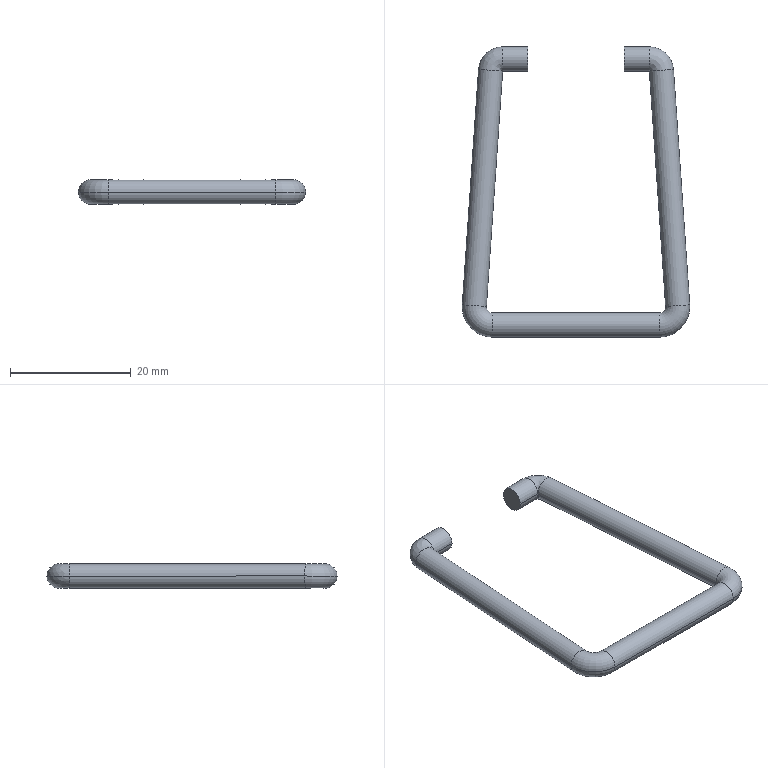Part | SolidWorks | features BaseBody 1 | 1 solid | 20 faces | box 37.633 x 48 x 4 mm | volume 1632 mm3 | cylinder 10 | spline 4 | torus 4 | plane 2 | commonest cylinder face diameters 4 x10
STEP:
#1=CARTESIAN_POINT('',(7.97,24.,0.));
#2=VERTEX_POINT('',#1);
#3=CARTESIAN_POINT('',(7.97,20.,0.));
#4=VERTEX_POINT('',#3);
#5=CARTESIAN_POINT('',(7.97,22.,0.));
#6=DIRECTION('',(-1.,0.,0.));
#7=DIRECTION('',(0.,1.,0.));
#8=AXIS2_PLACEMENT_3D('',#5,#6,#7);
#9=CIRCLE('',#8,2.);
#10=EDGE_CURVE('',#2,#4,#9,.T.);
#11=ORIENTED_EDGE('',*,*,#10,.T.);
#12=CARTESIAN_POINT('',(7.97,22.,0.));
#13=DIRECTION('',(-1.,0.,0.));
#14=DIRECTION('',(0.,-1.,0.));
#15=AXIS2_PLACEMENT_3D('',#12,#13,#14);
#16=CIRCLE('',#15,2.);
#17=EDGE_CURVE('',#4,#2,#16,.T.);
#18=ORIENTED_EDGE('',*,*,#17,.T.);
#19=EDGE_LOOP('',(#11,#18));
#20=FACE_OUTER_BOUND('',#19,.T.);
#21=CARTESIAN_POINT('',(7.97,22.,0.));
#22=DIRECTION('',(-1.,0.,0.));
#23=DIRECTION('',(0.,0.,1.));
#24=AXIS2_PLACEMENT_3D('',#21,#22,#23);
#25=PLANE('',#24);
#26=ADVANCED_FACE('',(#20),#25,.T.);
#27=CARTESIAN_POINT('',(12.109,20.,0.));
#28=VERTEX_POINT('',#27);
#29=CARTESIAN_POINT('',(12.109,20.,0.));
#30=DIRECTION('',(-1.,0.,0.));
#31=VECTOR('',#30,1000.);
#32=LINE('',#29,#31);
#33=EDGE_CURVE('',#28,#4,#32,.T.);
#34=ORIENTED_EDGE('',*,*,#33,.T.);
#35=ORIENTED_EDGE('',*,*,#10,.F.);
#36=CARTESIAN_POINT('',(12.109,24.,0.));
#37=VERTEX_POINT('',#36);
#38=CARTESIAN_POINT('',(12.109,24.,0.));
#39=DIRECTION('',(-1.,0.,0.));
#40=VECTOR('',#39,1000.);
#41=LINE('',#38,#40);
#42=EDGE_CURVE('',#37,#2,#41,.T.);
#43=ORIENTED_EDGE('',*,*,#42,.F.);
#44=CARTESIAN_POINT('',(12.109,22.,0.));
#45=DIRECTION('',(-1.,0.,0.));
#46=DIRECTION('',(0.,1.,0.));
#47=AXIS2_PLACEMENT_3D('',#44,#45,#46);
#48=CIRCLE('',#47,2.);
#49=EDGE_CURVE('',#37,#28,#48,.T.);
#50=ORIENTED_EDGE('',*,*,#49,.T.);
#51=EDGE_LOOP('',(#34,#35,#43,#50));
#52=FACE_OUTER_BOUND('',#51,.T.);
#53=CARTESIAN_POINT('',(12.109,22.,0.));
#54=DIRECTION('',(-1.,0.,0.));
#55=DIRECTION('',(0.,-1.,0.));
#56=AXIS2_PLACEMENT_3D('',#53,#54,#55);
#57=CYLINDRICAL_SURFACE('',#56,2.);
#58=ADVANCED_FACE('',(#52),#57,.T.);
#59=ORIENTED_EDGE('',*,*,#42,.T.);
#60=ORIENTED_EDGE('',*,*,#17,.F.);
#61=ORIENTED_EDGE('',*,*,#33,.F.);
#62=CARTESIAN_POINT('',(12.109,22.,0.));
#63=DIRECTION('',(-1.,0.,0.));
#64=DIRECTION('',(0.,-1.,0.));
#65=AXIS2_PLACEMENT_3D('',#62,#63,#64);
#66=CIRCLE('',#65,2.);
#67=EDGE_CURVE('',#28,#37,#66,.T.);
#68=ORIENTED_EDGE('',*,*,#67,.T.);
#69=EDGE_LOOP('',(#59,#60,#61,#68));
#70=FACE_OUTER_BOUND('',#69,.T.);
#71=CARTESIAN_POINT('',(12.109,22.,0.));
#72=DIRECTION('',(-1.,0.,0.));
#73=DIRECTION('',(0.,-1.,0.));
#74=AXIS2_PLACEMENT_3D('',#71,#72,#73);
#75=CYLINDRICAL_SURFACE('',#74,2.);
#76=ADVANCED_FACE('',(#70),#75,.T.);
#77=CARTESIAN_POINT('',(16.1,20.275,0.));
#78=VERTEX_POINT('',#77);
#79=CARTESIAN_POINT('',(12.109,20.,0.));
#80=DIRECTION('',(0.,0.,1.));
#81=DIRECTION('',(0.9976,0.0687,0.));
#82=AXIS2_PLACEMENT_3D('',#79,#80,#81);
#83=CIRCLE('',#82,4.);
#84=EDGE_CURVE('',#78,#37,#83,.T.);
#85=ORIENTED_EDGE('',*,*,#84,.T.);
#86=ORIENTED_EDGE('',*,*,#67,.F.);
#87=CARTESIAN_POINT('',(14.105,20.137,0.));
#88=DIRECTION('',(-0.0687,0.9976,0.));
#89=DIRECTION('',(-0.9976,-0.0687,0.));
#90=AXIS2_PLACEMENT_3D('',#87,#88,#89);
#91=CIRCLE('',#90,2.);
#92=EDGE_CURVE('',#28,#78,#91,.T.);
#93=ORIENTED_EDGE('',*,*,#92,.T.);
#94=EDGE_LOOP('',(#85,#86,#93));
#95=FACE_OUTER_BOUND('',#94,.T.);
#96=CARTESIAN_POINT('',(16.102,20.155,-0.1256));
#97=CARTESIAN_POINT('',(16.178,20.158,1.073));
#98=CARTESIAN_POINT('',(15.37,20.126,1.961));
#99=CARTESIAN_POINT('',(14.171,20.08,1.999));
#100=CARTESIAN_POINT('',(12.971,20.033,2.037));
#101=CARTESIAN_POINT('',(12.109,20.,1.201));
#102=CARTESIAN_POINT('',(12.109,20.,0.));
#103=CARTESIAN_POINT('',(16.012,22.478,-0.1256));
#104=CARTESIAN_POINT('',(16.086,22.524,1.073));
#105=CARTESIAN_POINT('',(15.297,22.023,1.961));
#106=CARTESIAN_POINT('',(14.124,21.279,1.999));
#107=CARTESIAN_POINT('',(12.952,20.535,2.037));
#108=CARTESIAN_POINT('',(12.109,20.,1.201));
#109=CARTESIAN_POINT('',(12.109,20.,0.));
#110=CARTESIAN_POINT('',(14.313,24.064,-0.1256));
#111=CARTESIAN_POINT('',(14.355,24.141,1.073));
#112=CARTESIAN_POINT('',(13.909,23.319,1.961));
#113=CARTESIAN_POINT('',(13.247,22.098,1.999));
#114=CARTESIAN_POINT('',(12.585,20.877,2.037));
#115=CARTESIAN_POINT('',(12.109,20.,1.201));
#116=CARTESIAN_POINT('',(12.109,20.,0.));
#117=CARTESIAN_POINT('',(11.989,23.994,-0.1256));
#118=CARTESIAN_POINT('',(11.987,24.07,1.073));
#119=CARTESIAN_POINT('',(12.011,23.262,1.961));
#120=CARTESIAN_POINT('',(12.047,22.062,1.999));
#121=CARTESIAN_POINT('',(12.083,20.862,2.037));
#122=CARTESIAN_POINT('',(12.109,20.,1.201));
#123=CARTESIAN_POINT('',(12.109,20.,0.));
#124=(BOUNDED_SURFACE()B_SPLINE_SURFACE(3,3,((#96,#97,#98,#99,#100,#101,#102),(#103,#104,#105,#106,#107,#108,#109),(#110,#111,#112,#113,#114,#115,#116),(#117,#118,#119,#120,#121,#122,#123)),.UNSPECIFIED.,.F.,.F.,.T.)B_SPLINE_SURFACE_WITH_KNOTS((4,4),(4,3,4),(0.,1.),(0.,1.,2.),.UNSPECIFIED.)GEOMETRIC_REPRESENTATION_ITEM()RATIONAL_B_SPLINE_SURFACE(((1.379,1.1,1.1,1.379,1.1,1.1,1.379),(1.113,0.8871,0.8871,1.113,0.8871,0.8871,1.113),(1.113,0.8871,0.8871,1.113,0.8871,0.8871,1.113),(1.379,1.1,1.1,1.379,1.1,1.1,1.379)))REPRESENTATION_ITEM('')SURFACE());
#125=ADVANCED_FACE('',(#95),#124,.T.);
#126=ORIENTED_EDGE('',*,*,#49,.F.);
#127=ORIENTED_EDGE('',*,*,#84,.F.);
#128=CARTESIAN_POINT('',(14.105,20.137,0.));
#129=DIRECTION('',(-0.0687,0.9976,0.));
#130=DIRECTION('',(0.9976,0.0687,0.));
#131=AXIS2_PLACEMENT_3D('',#128,#129,#130);
#132=CIRCLE('',#131,2.);
#133=EDGE_CURVE('',#78,#28,#132,.T.);
#134=ORIENTED_EDGE('',*,*,#133,.T.);
#135=EDGE_LOOP('',(#126,#127,#134));
#136=FACE_OUTER_BOUND('',#135,.T.);
#137=CARTESIAN_POINT('',(12.109,20.,0.));
#138=CARTESIAN_POINT('',(12.109,20.,-1.201));
#139=CARTESIAN_POINT('',(12.971,20.033,-2.037));
#140=CARTESIAN_POINT('',(14.171,20.08,-1.999));
#141=CARTESIAN_POINT('',(15.37,20.126,-1.961));
#142=CARTESIAN_POINT('',(16.178,20.158,-1.073));
#143=CARTESIAN_POINT('',(16.102,20.155,0.1256));
#144=CARTESIAN_POINT('',(12.109,20.,0.));
#145=CARTESIAN_POINT('',(12.109,20.,-1.201));
#146=CARTESIAN_POINT('',(12.952,20.535,-2.037));
#147=CARTESIAN_POINT('',(14.124,21.279,-1.999));
#148=CARTESIAN_POINT('',(15.297,22.023,-1.961));
#149=CARTESIAN_POINT('',(16.086,22.524,-1.073));
#150=CARTESIAN_POINT('',(16.012,22.478,0.1256));
#151=CARTESIAN_POINT('',(12.109,20.,0.));
#152=CARTESIAN_POINT('',(12.109,20.,-1.201));
#153=CARTESIAN_POINT('',(12.585,20.877,-2.037));
#154=CARTESIAN_POINT('',(13.247,22.098,-1.999));
#155=CARTESIAN_POINT('',(13.909,23.319,-1.961));
#156=CARTESIAN_POINT('',(14.355,24.141,-1.073));
#157=CARTESIAN_POINT('',(14.313,24.064,0.1256));
#158=CARTESIAN_POINT('',(12.109,20.,0.));
#159=CARTESIAN_POINT('',(12.109,20.,-1.201));
#160=CARTESIAN_POINT('',(12.083,20.862,-2.037));
#161=CARTESIAN_POINT('',(12.047,22.062,-1.999));
#162=CARTESIAN_POINT('',(12.011,23.262,-1.961));
#163=CARTESIAN_POINT('',(11.987,24.07,-1.073));
#164=CARTESIAN_POINT('',(11.989,23.994,0.1256));
#165=(BOUNDED_SURFACE()B_SPLINE_SURFACE(3,3,((#137,#138,#139,#140,#141,#142,#143),(#144,#145,#146,#147,#148,#149,#150),(#151,#152,#153,#154,#155,#156,#157),(#158,#159,#160,#161,#162,#163,#164)),.UNSPECIFIED.,.F.,.F.,.T.)B_SPLINE_SURFACE_WITH_KNOTS((4,4),(4,3,4),(0.,1.),(0.,1.,2.),.UNSPECIFIED.)GEOMETRIC_REPRESENTATION_ITEM()RATIONAL_B_SPLINE_SURFACE(((1.379,1.1,1.1,1.379,1.1,1.1,1.379),(1.113,0.8871,0.8871,1.113,0.8871,0.8871,1.113),(1.113,0.8871,0.8871,1.113,0.8871,0.8871,1.113),(1.379,1.1,1.1,1.379,1.1,1.1,1.379)))REPRESENTATION_ITEM('')SURFACE());
#166=ADVANCED_FACE('',(#136),#165,.T.);
#167=CARTESIAN_POINT('',(14.79,-18.931,0.));
#168=VERTEX_POINT('',#167);
#169=CARTESIAN_POINT('',(14.79,-18.931,0.));
#170=DIRECTION('',(-0.0687,0.9976,0.));
#171=VECTOR('',#170,1000.);
#172=LINE('',#169,#171);
#173=EDGE_CURVE('',#168,#28,#172,.T.);
#174=ORIENTED_EDGE('',*,*,#173,.T.);
#175=ORIENTED_EDGE('',*,*,#133,.F.);
#176=CARTESIAN_POINT('',(18.781,-18.656,0.));
#177=VERTEX_POINT('',#176);
#178=CARTESIAN_POINT('',(18.781,-18.656,0.));
#179=DIRECTION('',(-0.0687,0.9976,0.));
#180=VECTOR('',#179,1000.);
#181=LINE('',#178,#180);
#182=EDGE_CURVE('',#177,#78,#181,.T.);
#183=ORIENTED_EDGE('',*,*,#182,.F.);
#184=CARTESIAN_POINT('',(16.786,-18.794,0.));
#185=DIRECTION('',(-0.0687,0.9976,0.));
#186=DIRECTION('',(0.9976,0.0687,0.));
#187=AXIS2_PLACEMENT_3D('',#184,#185,#186);
#188=CIRCLE('',#187,2.);
#189=EDGE_CURVE('',#177,#168,#188,.T.);
#190=ORIENTED_EDGE('',*,*,#189,.T.);
#191=EDGE_LOOP('',(#174,#175,#183,#190));
#192=FACE_OUTER_BOUND('',#191,.T.);
#193=CARTESIAN_POINT('',(16.786,-18.794,0.));
#194=DIRECTION('',(-0.0687,0.9976,0.));
#195=DIRECTION('',(-0.9976,-0.0687,0.));
#196=AXIS2_PLACEMENT_3D('',#193,#194,#195);
#197=CYLINDRICAL_SURFACE('',#196,2.);
#198=ADVANCED_FACE('',(#192),#197,.T.);
#199=ORIENTED_EDGE('',*,*,#182,.T.);
#200=ORIENTED_EDGE('',*,*,#92,.F.);
#201=ORIENTED_EDGE('',*,*,#173,.F.);
#202=CARTESIAN_POINT('',(16.786,-18.794,0.));
#203=DIRECTION('',(-0.0687,0.9976,0.));
#204=DIRECTION('',(-0.9976,-0.0687,0.));
#205=AXIS2_PLACEMENT_3D('',#202,#203,#204);
#206=CIRCLE('',#205,2.);
#207=EDGE_CURVE('',#168,#177,#206,.T.);
#208=ORIENTED_EDGE('',*,*,#207,.T.);
#209=EDGE_LOOP('',(#199,#200,#201,#208));
#210=FACE_OUTER_BOUND('',#209,.T.);
#211=CARTESIAN_POINT('',(16.786,-18.794,0.));
#212=DIRECTION('',(-0.0687,0.9976,0.));
#213=DIRECTION('',(-0.9976,-0.0687,0.));
#214=AXIS2_PLACEMENT_3D('',#211,#212,#213);
#215=CYLINDRICAL_SURFACE('',#214,2.);
#216=ADVANCED_FACE('',(#210),#215,.T.);
#217=CARTESIAN_POINT('',(13.793,-24.,0.));
#218=VERTEX_POINT('',#217);
#219=CARTESIAN_POINT('',(13.793,-19.,0.));
#220=DIRECTION('',(0.,0.,1.));
#221=DIRECTION('',(0.,-1.,0.));
#222=AXIS2_PLACEMENT_3D('',#219,#220,#221);
#223=CIRCLE('',#222,5.);
#224=EDGE_CURVE('',#218,#177,#223,.T.);
#225=ORIENTED_EDGE('',*,*,#224,.T.);
#226=ORIENTED_EDGE('',*,*,#207,.F.);
#227=CARTESIAN_POINT('',(13.793,-20.,0.));
#228=VERTEX_POINT('',#227);
#229=CARTESIAN_POINT('',(13.793,-19.,0.));
#230=DIRECTION('',(0.,0.,1.));
#231=DIRECTION('',(0.,-1.,0.));
#232=AXIS2_PLACEMENT_3D('',#229,#230,#231);
#233=CIRCLE('',#232,1.);
#234=EDGE_CURVE('',#228,#168,#233,.T.);
#235=ORIENTED_EDGE('',*,*,#234,.F.);
#236=CARTESIAN_POINT('',(13.793,-22.,0.));
#237=DIRECTION('',(1.,0.,0.));
#238=DIRECTION('',(0.,1.,0.));
#239=AXIS2_PLACEMENT_3D('',#236,#237,#238);
#240=CIRCLE('',#239,2.);
#241=EDGE_CURVE('',#228,#218,#240,.T.);
#242=ORIENTED_EDGE('',*,*,#241,.T.);
#243=EDGE_LOOP('',(#225,#226,#235,#242));
#244=FACE_OUTER_BOUND('',#243,.T.);
#245=CARTESIAN_POINT('',(13.793,-19.,0.));
#246=DIRECTION('',(0.,0.,1.));
#247=DIRECTION('',(0.,1.,0.));
#248=AXIS2_PLACEMENT_3D('',#245,#246,#247);
#249=TOROIDAL_SURFACE('',#248,3.,2.);
#250=ADVANCED_FACE('',(#244),#249,.T.);
#251=ORIENTED_EDGE('',*,*,#234,.T.);
#252=ORIENTED_EDGE('',*,*,#189,.F.);
#253=ORIENTED_EDGE('',*,*,#224,.F.);
#254=CARTESIAN_POINT('',(13.793,-22.,0.));
#255=DIRECTION('',(1.,0.,0.));
#256=DIRECTION('',(0.,-1.,0.));
#257=AXIS2_PLACEMENT_3D('',#254,#255,#256);
#258=CIRCLE('',#257,2.);
#259=EDGE_CURVE('',#218,#228,#258,.T.);
#260=ORIENTED_EDGE('',*,*,#259,.T.);
#261=EDGE_LOOP('',(#251,#252,#253,#260));
#262=FACE_OUTER_BOUND('',#261,.T.);
#263=CARTESIAN_POINT('',(13.793,-19.,0.));
#264=DIRECTION('',(0.,0.,1.));
#265=DIRECTION('',(0.,1.,0.));
#266=AXIS2_PLACEMENT_3D('',#263,#264,#265);
#267=TOROIDAL_SURFACE('',#266,3.,2.);
#268=ADVANCED_FACE('',(#262),#267,.T.);
#269=CARTESIAN_POINT('',(-13.841,-20.,0.));
#270=VERTEX_POINT('',#269);
#271=CARTESIAN_POINT('',(-13.841,-20.,0.));
#272=DIRECTION('',(1.,0.,0.));
#273=VECTOR('',#272,1000.);
#274=LINE('',#271,#273);
#275=EDGE_CURVE('',#270,#228,#274,.T.);
#276=ORIENTED_EDGE('',*,*,#275,.T.);
#277=ORIENTED_EDGE('',*,*,#259,.F.);
#278=CARTESIAN_POINT('',(-13.841,-24.,0.));
#279=VERTEX_POINT('',#278);
#280=CARTESIAN_POINT('',(-13.841,-24.,0.));
#281=DIRECTION('',(1.,0.,0.));
#282=VECTOR('',#281,1000.);
#283=LINE('',#280,#282);
#284=EDGE_CURVE('',#279,#218,#283,.T.);
#285=ORIENTED_EDGE('',*,*,#284,.F.);
#286=CARTESIAN_POINT('',(-13.841,-22.,0.));
#287=DIRECTION('',(1.,0.,0.));
#288=DIRECTION('',(0.,-1.,0.));
#289=AXIS2_PLACEMENT_3D('',#286,#287,#288);
#290=CIRCLE('',#289,2.);
#291=EDGE_CURVE('',#279,#270,#290,.T.);
#292=ORIENTED_EDGE('',*,*,#291,.T.);
#293=EDGE_LOOP('',(#276,#277,#285,#292));
#294=FACE_OUTER_BOUND('',#293,.T.);
#295=CARTESIAN_POINT('',(-13.841,-22.,0.));
#296=DIRECTION('',(1.,0.,0.));
#297=DIRECTION('',(0.,1.,0.));
#298=AXIS2_PLACEMENT_3D('',#295,#296,#297);
#299=CYLINDRICAL_SURFACE('',#298,2.);
#300=ADVANCED_FACE('',(#294),#299,.T.);
#301=ORIENTED_EDGE('',*,*,#284,.T.);
#302=ORIENTED_EDGE('',*,*,#241,.F.);
#303=ORIENTED_EDGE('',*,*,#275,.F.);
#304=CARTESIAN_POINT('',(-13.841,-22.,0.));
#305=DIRECTION('',(1.,0.,0.));
#306=DIRECTION('',(0.,1.,0.));
#307=AXIS2_PLACEMENT_3D('',#304,#305,#306);
#308=CIRCLE('',#307,2.);
#309=EDGE_CURVE('',#270,#279,#308,.T.);
#310=ORIENTED_EDGE('',*,*,#309,.T.);
#311=EDGE_LOOP('',(#301,#302,#303,#310));
#312=FACE_OUTER_BOUND('',#311,.T.);
#313=CARTESIAN_POINT('',(-13.841,-22.,0.));
#314=DIRECTION('',(1.,0.,0.));
#315=DIRECTION('',(0.,1.,0.));
#316=AXIS2_PLACEMENT_3D('',#313,#314,#315);
#317=CYLINDRICAL_SURFACE('',#316,2.);
#318=ADVANCED_FACE('',(#312),#317,.T.);
#319=CARTESIAN_POINT('',(-18.829,-18.656,0.));
#320=VERTEX_POINT('',#319);
#321=CARTESIAN_POINT('',(-13.841,-19.,0.));
#322=DIRECTION('',(0.,0.,1.));
#323=DIRECTION('',(-0.9976,0.0687,0.));
#324=AXIS2_PLACEMENT_3D('',#321,#322,#323);
#325=CIRCLE('',#324,5.);
#326=EDGE_CURVE('',#320,#279,#325,.T.);
#327=ORIENTED_EDGE('',*,*,#326,.T.);
#328=ORIENTED_EDGE('',*,*,#309,.F.);
#329=CARTESIAN_POINT('',(-14.838,-18.931,0.));
#330=VERTEX_POINT('',#329);
#331=CARTESIAN_POINT('',(-13.841,-19.,0.));
#332=DIRECTION('',(0.,0.,1.));
#333=DIRECTION('',(-0.9976,0.0687,0.));
#334=AXIS2_PLACEMENT_3D('',#331,#332,#333);
#335=CIRCLE('',#334,1.);
#336=EDGE_CURVE('',#330,#270,#335,.T.);
#337=ORIENTED_EDGE('',*,*,#336,.F.);
#338=CARTESIAN_POINT('',(-16.834,-18.794,0.));
#339=DIRECTION('',(-0.0687,-0.9976,0.));
#340=DIRECTION('',(0.9976,-0.0687,0.));
#341=AXIS2_PLACEMENT_3D('',#338,#339,#340);
#342=CIRCLE('',#341,2.);
#343=EDGE_CURVE('',#330,#320,#342,.T.);
#344=ORIENTED_EDGE('',*,*,#343,.T.);
#345=EDGE_LOOP('',(#327,#328,#337,#344));
#346=FACE_OUTER_BOUND('',#345,.T.);
#347=CARTESIAN_POINT('',(-13.841,-19.,0.));
#348=DIRECTION('',(0.,0.,1.));
#349=DIRECTION('',(0.9976,-0.0687,0.));
#350=AXIS2_PLACEMENT_3D('',#347,#348,#349);
#351=TOROIDAL_SURFACE('',#350,3.,2.);
#352=ADVANCED_FACE('',(#346),#351,.T.);
#353=ORIENTED_EDGE('',*,*,#336,.T.);
#354=ORIENTED_EDGE('',*,*,#291,.F.);
#355=ORIENTED_EDGE('',*,*,#326,.F.);
#356=CARTESIAN_POINT('',(-16.834,-18.794,0.));
#357=DIRECTION('',(-0.0687,-0.9976,0.));
#358=DIRECTION('',(-0.9976,0.0687,0.));
#359=AXIS2_PLACEMENT_3D('',#356,#357,#358);
#360=CIRCLE('',#359,2.);
#361=EDGE_CURVE('',#320,#330,#360,.T.);
#362=ORIENTED_EDGE('',*,*,#361,.T.);
#363=EDGE_LOOP('',(#353,#354,#355,#362));
#364=FACE_OUTER_BOUND('',#363,.T.);
#365=CARTESIAN_POINT('',(-13.841,-19.,0.));
#366=DIRECTION('',(0.,0.,1.));
#367=DIRECTION('',(0.9976,-0.0687,0.));
#368=AXIS2_PLACEMENT_3D('',#365,#366,#367);
#369=TOROIDAL_SURFACE('',#368,3.,2.);
#370=ADVANCED_FACE('',(#364),#369,.T.);
#371=CARTESIAN_POINT('',(-12.157,20.,0.));
#372=VERTEX_POINT('',#371);
#373=CARTESIAN_POINT('',(-12.157,20.,0.));
#374=DIRECTION('',(-0.0687,-0.9976,0.));
#375=VECTOR('',#374,1000.);
#376=LINE('',#373,#375);
#377=EDGE_CURVE('',#372,#330,#376,.T.);
#378=ORIENTED_EDGE('',*,*,#377,.T.);
#379=ORIENTED_EDGE('',*,*,#361,.F.);
#380=CARTESIAN_POINT('',(-16.148,20.275,0.));
#381=VERTEX_POINT('',#380);
#382=CARTESIAN_POINT('',(-16.148,20.275,0.));
#383=DIRECTION('',(-0.0687,-0.9976,0.));
#384=VECTOR('',#383,1000.);
#385=LINE('',#382,#384);
#386=EDGE_CURVE('',#381,#320,#385,.T.);
#387=ORIENTED_EDGE('',*,*,#386,.F.);
#388=CARTESIAN_POINT('',(-14.153,20.137,0.));
#389=DIRECTION('',(-0.0687,-0.9976,0.));
#390=DIRECTION('',(-0.9976,0.0687,0.));
#391=AXIS2_PLACEMENT_3D('',#388,#389,#390);
#392=CIRCLE('',#391,2.);
#393=EDGE_CURVE('',#381,#372,#392,.T.);
#394=ORIENTED_EDGE('',*,*,#393,.T.);
#395=EDGE_LOOP('',(#378,#379,#387,#394));
#396=FACE_OUTER_BOUND('',#395,.T.);
#397=CARTESIAN_POINT('',(-14.153,20.137,0.));
#398=DIRECTION('',(-0.0687,-0.9976,0.));
#399=DIRECTION('',(0.9976,-0.0687,0.));
#400=AXIS2_PLACEMENT_3D('',#397,#398,#399);
#401=CYLINDRICAL_SURFACE('',#400,2.);
#402=ADVANCED_FACE('',(#396),#401,.T.);
#403=ORIENTED_EDGE('',*,*,#386,.T.);
#404=ORIENTED_EDGE('',*,*,#343,.F.);
#405=ORIENTED_EDGE('',*,*,#377,.F.);
#406=CARTESIAN_POINT('',(-14.153,20.137,0.));
#407=DIRECTION('',(-0.0687,-0.9976,0.));
#408=DIRECTION('',(0.9976,-0.0687,0.));
#409=AXIS2_PLACEMENT_3D('',#406,#407,#408);
#410=CIRCLE('',#409,2.);
#411=EDGE_CURVE('',#372,#381,#410,.T.);
#412=ORIENTED_EDGE('',*,*,#411,.T.);
#413=EDGE_LOOP('',(#403,#404,#405,#412));
#414=FACE_OUTER_BOUND('',#413,.T.);
#415=CARTESIAN_POINT('',(-14.153,20.137,0.));
#416=DIRECTION('',(-0.0687,-0.9976,0.));
#417=DIRECTION('',(0.9976,-0.0687,0.));
#418=AXIS2_PLACEMENT_3D('',#415,#416,#417);
#419=CYLINDRICAL_SURFACE('',#418,2.);
#420=ADVANCED_FACE('',(#414),#419,.T.);
#421=CARTESIAN_POINT('',(-12.157,24.,0.));
#422=VERTEX_POINT('',#421);
#423=CARTESIAN_POINT('',(-12.157,20.,0.));
#424=DIRECTION('',(0.,0.,1.));
#425=DIRECTION('',(0.,1.,0.));
#426=AXIS2_PLACEMENT_3D('',#423,#424,#425);
#427=CIRCLE('',#426,4.);
#428=EDGE_CURVE('',#422,#381,#427,.T.);
#429=ORIENTED_EDGE('',*,*,#428,.T.);
#430=ORIENTED_EDGE('',*,*,#411,.F.);
#431=CARTESIAN_POINT('',(-12.157,22.,0.));
#432=DIRECTION('',(-1.,0.,0.));
#433=DIRECTION('',(0.,-1.,0.));
#434=AXIS2_PLACEMENT_3D('',#431,#432,#433);
#435=CIRCLE('',#434,2.);
#436=EDGE_CURVE('',#372,#422,#435,.T.);
#437=ORIENTED_EDGE('',*,*,#436,.T.);
#438=EDGE_LOOP('',(#429,#430,#437));
#439=FACE_OUTER_BOUND('',#438,.T.);
#440=CARTESIAN_POINT('',(-12.037,23.994,-0.1256));
#441=CARTESIAN_POINT('',(-12.035,24.07,1.073));
#442=CARTESIAN_POINT('',(-12.059,23.262,1.961));
#443=CARTESIAN_POINT('',(-12.095,22.062,1.999));
#444=CARTESIAN_POINT('',(-12.131,20.862,2.037));
#445=CARTESIAN_POINT('',(-12.157,20.,1.201));
#446=CARTESIAN_POINT('',(-12.157,20.,0.));
#447=CARTESIAN_POINT('',(-14.361,24.064,-0.1256));
#448=CARTESIAN_POINT('',(-14.403,24.141,1.073));
#449=CARTESIAN_POINT('',(-13.957,23.319,1.961));
#450=CARTESIAN_POINT('',(-13.295,22.098,1.999));
#451=CARTESIAN_POINT('',(-12.633,20.877,2.037));
#452=CARTESIAN_POINT('',(-12.157,20.,1.201));
#453=CARTESIAN_POINT('',(-12.157,20.,0.));
#454=CARTESIAN_POINT('',(-16.06,22.478,-0.1256));
#455=CARTESIAN_POINT('',(-16.134,22.524,1.073));
#456=CARTESIAN_POINT('',(-15.345,22.023,1.961));
#457=CARTESIAN_POINT('',(-14.172,21.279,1.999));
#458=CARTESIAN_POINT('',(-13.,20.535,2.037));
#459=CARTESIAN_POINT('',(-12.157,20.,1.201));
#460=CARTESIAN_POINT('',(-12.157,20.,0.));
#461=CARTESIAN_POINT('',(-16.15,20.155,-0.1256));
#462=CARTESIAN_POINT('',(-16.226,20.158,1.073));
#463=CARTESIAN_POINT('',(-15.418,20.126,1.961));
#464=CARTESIAN_POINT('',(-14.219,20.08,1.999));
#465=CARTESIAN_POINT('',(-13.019,20.033,2.037));
#466=CARTESIAN_POINT('',(-12.157,20.,1.201));
#467=CARTESIAN_POINT('',(-12.157,20.,0.));
#468=(BOUNDED_SURFACE()B_SPLINE_SURFACE(3,3,((#440,#441,#442,#443,#444,#445,#446),(#447,#448,#449,#450,#451,#452,#453),(#454,#455,#456,#457,#458,#459,#460),(#461,#462,#463,#464,#465,#466,#467)),.UNSPECIFIED.,.F.,.F.,.T.)B_SPLINE_SURFACE_WITH_KNOTS((4,4),(4,3,4),(0.,1.),(0.,1.,2.),.UNSPECIFIED.)GEOMETRIC_REPRESENTATION_ITEM()RATIONAL_B_SPLINE_SURFACE(((1.379,1.1,1.1,1.379,1.1,1.1,1.379),(1.113,0.8871,0.8871,1.113,0.8871,0.8871,1.113),(1.113,0.8871,0.8871,1.113,0.8871,0.8871,1.113),(1.379,1.1,1.1,1.379,1.1,1.1,1.379)))REPRESENTATION_ITEM('')SURFACE());
#469=ADVANCED_FACE('',(#439),#468,.T.);
#470=ORIENTED_EDGE('',*,*,#393,.F.);
#471=ORIENTED_EDGE('',*,*,#428,.F.);
#472=CARTESIAN_POINT('',(-12.157,22.,0.));
#473=DIRECTION('',(-1.,0.,0.));
#474=DIRECTION('',(0.,1.,0.));
#475=AXIS2_PLACEMENT_3D('',#472,#473,#474);
#476=CIRCLE('',#475,2.);
#477=EDGE_CURVE('',#422,#372,#476,.T.);
#478=ORIENTED_EDGE('',*,*,#477,.T.);
#479=EDGE_LOOP('',(#470,#471,#478));
#480=FACE_OUTER_BOUND('',#479,.T.);
#481=CARTESIAN_POINT('',(-12.157,20.,0.));
#482=CARTESIAN_POINT('',(-12.157,20.,-1.201));
#483=CARTESIAN_POINT('',(-12.131,20.862,-2.037));
#484=CARTESIAN_POINT('',(-12.095,22.062,-1.999));
#485=CARTESIAN_POINT('',(-12.059,23.262,-1.961));
#486=CARTESIAN_POINT('',(-12.035,24.07,-1.073));
#487=CARTESIAN_POINT('',(-12.037,23.994,0.1256));
#488=CARTESIAN_POINT('',(-12.157,20.,0.));
#489=CARTESIAN_POINT('',(-12.157,20.,-1.201));
#490=CARTESIAN_POINT('',(-12.633,20.877,-2.037));
#491=CARTESIAN_POINT('',(-13.295,22.098,-1.999));
#492=CARTESIAN_POINT('',(-13.957,23.319,-1.961));
#493=CARTESIAN_POINT('',(-14.403,24.141,-1.073));
#494=CARTESIAN_POINT('',(-14.361,24.064,0.1256));
#495=CARTESIAN_POINT('',(-12.157,20.,0.));
#496=CARTESIAN_POINT('',(-12.157,20.,-1.201));
#497=CARTESIAN_POINT('',(-13.,20.535,-2.037));
#498=CARTESIAN_POINT('',(-14.172,21.279,-1.999));
#499=CARTESIAN_POINT('',(-15.345,22.023,-1.961));
#500=CARTESIAN_POINT('',(-16.134,22.524,-1.073));
#501=CARTESIAN_POINT('',(-16.06,22.478,0.1256));
#502=CARTESIAN_POINT('',(-12.157,20.,0.));
#503=CARTESIAN_POINT('',(-12.157,20.,-1.201));
#504=CARTESIAN_POINT('',(-13.019,20.033,-2.037));
#505=CARTESIAN_POINT('',(-14.219,20.08,-1.999));
#506=CARTESIAN_POINT('',(-15.418,20.126,-1.961));
#507=CARTESIAN_POINT('',(-16.226,20.158,-1.073));
#508=CARTESIAN_POINT('',(-16.15,20.155,0.1256));
#509=(BOUNDED_SURFACE()B_SPLINE_SURFACE(3,3,((#481,#482,#483,#484,#485,#486,#487),(#488,#489,#490,#491,#492,#493,#494),(#495,#496,#497,#498,#499,#500,#501),(#502,#503,#504,#505,#506,#507,#508)),.UNSPECIFIED.,.F.,.F.,.T.)B_SPLINE_SURFACE_WITH_KNOTS((4,4),(4,3,4),(0.,1.),(0.,1.,2.),.UNSPECIFIED.)GEOMETRIC_REPRESENTATION_ITEM()RATIONAL_B_SPLINE_SURFACE(((1.379,1.1,1.1,1.379,1.1,1.1,1.379),(1.113,0.8871,0.8871,1.113,0.8871,0.8871,1.113),(1.113,0.8871,0.8871,1.113,0.8871,0.8871,1.113),(1.379,1.1,1.1,1.379,1.1,1.1,1.379)))REPRESENTATION_ITEM('')SURFACE());
#510=ADVANCED_FACE('',(#480),#509,.T.);
#511=CARTESIAN_POINT('',(-7.97,20.,0.));
#512=VERTEX_POINT('',#511);
#513=CARTESIAN_POINT('',(-7.97,20.,0.));
#514=DIRECTION('',(-1.,0.,0.));
#515=VECTOR('',#514,1000.);
#516=LINE('',#513,#515);
#517=EDGE_CURVE('',#512,#372,#516,.T.);
#518=ORIENTED_EDGE('',*,*,#517,.T.);
#519=ORIENTED_EDGE('',*,*,#477,.F.);
#520=CARTESIAN_POINT('',(-7.97,24.,0.));
#521=VERTEX_POINT('',#520);
#522=CARTESIAN_POINT('',(-7.97,24.,0.));
#523=DIRECTION('',(-1.,0.,0.));
#524=VECTOR('',#523,1000.);
#525=LINE('',#522,#524);
#526=EDGE_CURVE('',#521,#422,#525,.T.);
#527=ORIENTED_EDGE('',*,*,#526,.F.);
#528=CARTESIAN_POINT('',(-7.97,22.,0.));
#529=DIRECTION('',(-1.,0.,0.));
#530=DIRECTION('',(0.,1.,0.));
#531=AXIS2_PLACEMENT_3D('',#528,#529,#530);
#532=CIRCLE('',#531,2.);
#533=EDGE_CURVE('',#521,#512,#532,.T.);
#534=ORIENTED_EDGE('',*,*,#533,.T.);
#535=EDGE_LOOP('',(#518,#519,#527,#534));
#536=FACE_OUTER_BOUND('',#535,.T.);
#537=CARTESIAN_POINT('',(-7.97,22.,0.));
#538=DIRECTION('',(-1.,0.,0.));
#539=DIRECTION('',(0.,-1.,0.));
#540=AXIS2_PLACEMENT_3D('',#537,#538,#539);
#541=CYLINDRICAL_SURFACE('',#540,2.);
#542=ADVANCED_FACE('',(#536),#541,.T.);
#543=ORIENTED_EDGE('',*,*,#526,.T.);
#544=ORIENTED_EDGE('',*,*,#436,.F.);
#545=ORIENTED_EDGE('',*,*,#517,.F.);
#546=CARTESIAN_POINT('',(-7.97,22.,0.));
#547=DIRECTION('',(-1.,0.,0.));
#548=DIRECTION('',(0.,-1.,0.));
#549=AXIS2_PLACEMENT_3D('',#546,#547,#548);
#550=CIRCLE('',#549,2.);
#551=EDGE_CURVE('',#512,#521,#550,.T.);
#552=ORIENTED_EDGE('',*,*,#551,.T.);
#553=EDGE_LOOP('',(#543,#544,#545,#552));
#554=FACE_OUTER_BOUND('',#553,.T.);
#555=CARTESIAN_POINT('',(-7.97,22.,0.));
#556=DIRECTION('',(-1.,0.,0.));
#557=DIRECTION('',(0.,-1.,0.));
#558=AXIS2_PLACEMENT_3D('',#555,#556,#557);
#559=CYLINDRICAL_SURFACE('',#558,2.);
#560=ADVANCED_FACE('',(#554),#559,.T.);
#561=ORIENTED_EDGE('',*,*,#533,.F.);
#562=ORIENTED_EDGE('',*,*,#551,.F.);
#563=EDGE_LOOP('',(#561,#562));
#564=FACE_OUTER_BOUND('',#563,.T.);
#565=CARTESIAN_POINT('',(-7.97,22.,0.));
#566=DIRECTION('',(-1.,0.,0.));
#567=DIRECTION('',(0.,0.,1.));
#568=AXIS2_PLACEMENT_3D('',#565,#566,#567);
#569=PLANE('',#568);
#570=ADVANCED_FACE('',(#564),#569,.F.);
#571=CLOSED_SHELL('',(#26,#58,#76,#125,#166,#198,#216,#250,#268,#300,#318,#352,#370,#402,#420,#469,#510,#542,#560,#570));
#572=MANIFOLD_SOLID_BREP('',#571);
#573=CARTESIAN_POINT('',(0.,0.,0.));
#574=DIRECTION('',(0.,0.,1.));
#575=DIRECTION('',(1.,0.,0.));
#576=AXIS2_PLACEMENT_3D('',#573,#574,#575);
#577=(LENGTH_UNIT()NAMED_UNIT(*)SI_UNIT(.MILLI.,.METRE.));
#578=UNCERTAINTY_MEASURE_WITH_UNIT(LENGTH_MEASURE(0.00001),#577,'','');
#579=(NAMED_UNIT(*)PLANE_ANGLE_UNIT()SI_UNIT($,.RADIAN.));
#580=(NAMED_UNIT(*)SI_UNIT($,.STERADIAN.)SOLID_ANGLE_UNIT());
#581=(GEOMETRIC_REPRESENTATION_CONTEXT(3)GLOBAL_UNCERTAINTY_ASSIGNED_CONTEXT((#578))GLOBAL_UNIT_ASSIGNED_CONTEXT((#577,#579,#580))REPRESENTATION_CONTEXT('',''));
#582=ADVANCED_BREP_SHAPE_REPRESENTATION('',(#572,#576),#581);